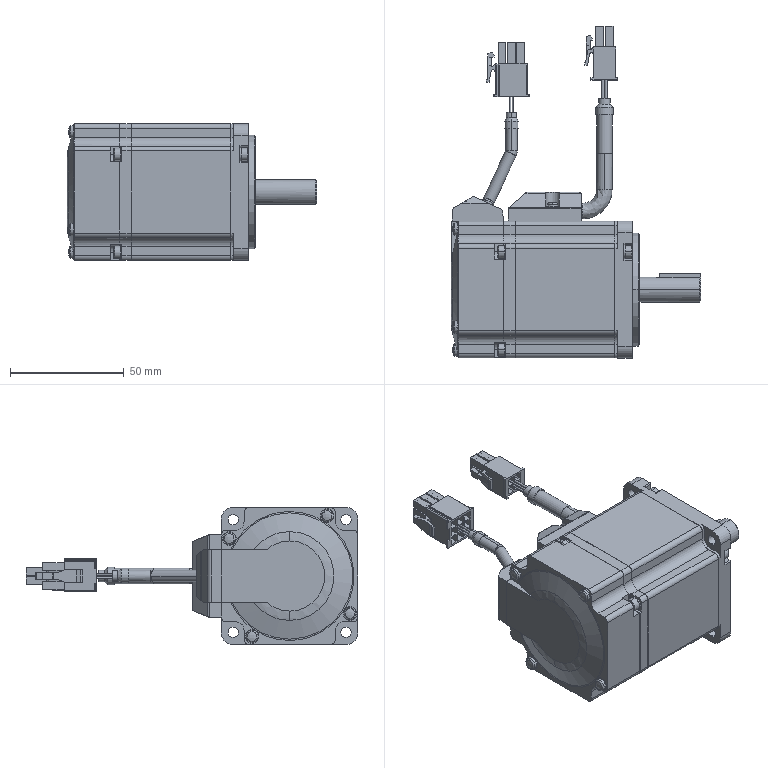Part | SolidWorks | features BaseBody 7 | 7 solids | 956 faces | box 109.5 x 145.682 x 60 mm | volume 283443 mm3 | plane 555 | cylinder 302 | cone 61 | spline 34 | torus 4 | commonest cylinder face diameters 1 x35 4 x34 6 x29 2.6 x26 3.92 x20 5.5 x16